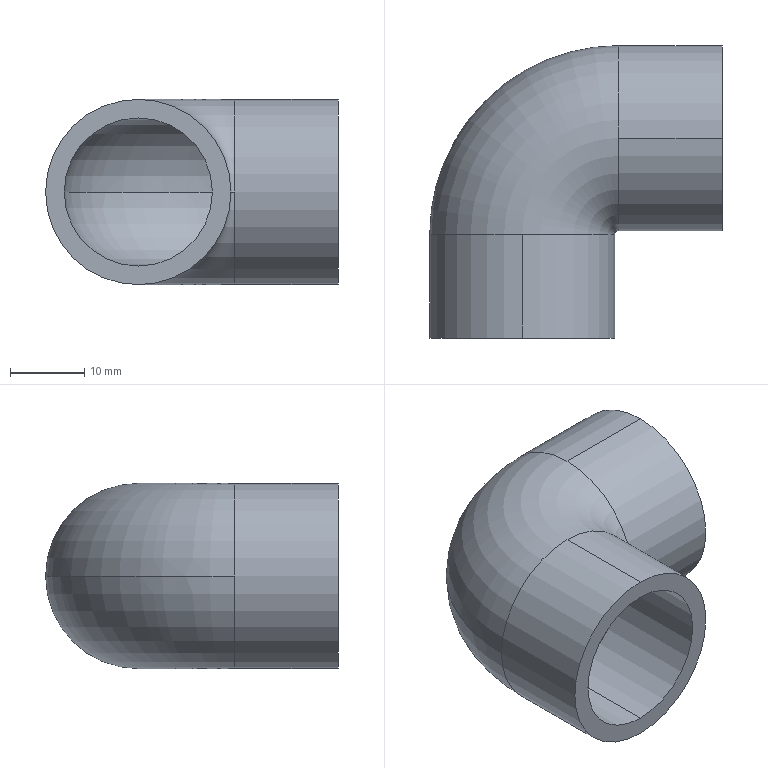Part | SolidWorks | features Sweep 1 | 1 solid | 14 faces | box 39.5 x 39.5 x 25 mm | volume 8557 mm3 | cylinder 8 | torus 4 | plane 2 | commonest cylinder face diameters 20 x4 25 x4
STEP:
#1=CARTESIAN_POINT('',(-10.,14.,0.));
#2=VERTEX_POINT('',#1);
#3=CARTESIAN_POINT('',(0.,14.,10.));
#4=VERTEX_POINT('',#3);
#5=CARTESIAN_POINT('',(0.,14.,0.));
#6=DIRECTION('',(0.,1.,0.));
#7=DIRECTION('',(0.,0.,1.));
#8=AXIS2_PLACEMENT_3D('',#5,#6,#7);
#9=CIRCLE('',#8,10.);
#10=EDGE_CURVE('',#2,#4,#9,.T.);
#11=ORIENTED_EDGE('',*,*,#10,.F.);
#12=CARTESIAN_POINT('',(13.,37.,0.));
#13=VERTEX_POINT('',#12);
#14=CARTESIAN_POINT('',(13.,14.,0.));
#15=DIRECTION('',(0.,0.,-1.));
#16=DIRECTION('',(-1.,0.,0.));
#17=AXIS2_PLACEMENT_3D('',#14,#15,#16);
#18=CIRCLE('',#17,23.);
#19=EDGE_CURVE('',#2,#13,#18,.T.);
#20=ORIENTED_EDGE('',*,*,#19,.T.);
#21=CARTESIAN_POINT('',(13.,27.,10.));
#22=VERTEX_POINT('',#21);
#23=CARTESIAN_POINT('',(13.,27.,0.));
#24=DIRECTION('',(1.,0.,0.));
#25=DIRECTION('',(0.,0.,1.));
#26=AXIS2_PLACEMENT_3D('',#23,#24,#25);
#27=CIRCLE('',#26,10.);
#28=EDGE_CURVE('',#13,#22,#27,.T.);
#29=ORIENTED_EDGE('',*,*,#28,.T.);
#30=CARTESIAN_POINT('',(13.,17.,0.));
#31=VERTEX_POINT('',#30);
#32=CARTESIAN_POINT('',(13.,27.,0.));
#33=DIRECTION('',(1.,0.,0.));
#34=DIRECTION('',(0.,0.,1.));
#35=AXIS2_PLACEMENT_3D('',#32,#33,#34);
#36=CIRCLE('',#35,10.);
#37=EDGE_CURVE('',#22,#31,#36,.T.);
#38=ORIENTED_EDGE('',*,*,#37,.T.);
#39=CARTESIAN_POINT('',(10.,14.,0.));
#40=VERTEX_POINT('',#39);
#41=CARTESIAN_POINT('',(13.,14.,0.));
#42=DIRECTION('',(0.,0.,-1.));
#43=DIRECTION('',(-1.,0.,0.));
#44=AXIS2_PLACEMENT_3D('',#41,#42,#43);
#45=CIRCLE('',#44,3.);
#46=EDGE_CURVE('',#40,#31,#45,.T.);
#47=ORIENTED_EDGE('',*,*,#46,.F.);
#48=CARTESIAN_POINT('',(0.,14.,0.));
#49=DIRECTION('',(0.,1.,0.));
#50=DIRECTION('',(0.,0.,1.));
#51=AXIS2_PLACEMENT_3D('',#48,#49,#50);
#52=CIRCLE('',#51,10.);
#53=EDGE_CURVE('',#4,#40,#52,.T.);
#54=ORIENTED_EDGE('',*,*,#53,.F.);
#55=EDGE_LOOP('',(#11,#20,#29,#38,#47,#54));
#56=FACE_OUTER_BOUND('',#55,.T.);
#57=CARTESIAN_POINT('',(13.,14.,0.));
#58=DIRECTION('',(0.,0.,-1.));
#59=DIRECTION('',(-1.,0.,0.));
#60=AXIS2_PLACEMENT_3D('',#57,#58,#59);
#61=TOROIDAL_SURFACE('',#60,13.,10.);
#62=ADVANCED_FACE('',(#56),#61,.F.);
#63=CARTESIAN_POINT('',(0.,14.,-12.5));
#64=VERTEX_POINT('',#63);
#65=CARTESIAN_POINT('',(-12.5,14.,0.));
#66=VERTEX_POINT('',#65);
#67=CARTESIAN_POINT('',(0.,14.,0.));
#68=DIRECTION('',(0.,1.,0.));
#69=DIRECTION('',(0.,0.,1.));
#70=AXIS2_PLACEMENT_3D('',#67,#68,#69);
#71=CIRCLE('',#70,12.5);
#72=EDGE_CURVE('',#64,#66,#71,.T.);
#73=ORIENTED_EDGE('',*,*,#72,.T.);
#74=CARTESIAN_POINT('',(13.,39.5,0.));
#75=VERTEX_POINT('',#74);
#76=CARTESIAN_POINT('',(13.,14.,0.));
#77=DIRECTION('',(0.,0.,-1.));
#78=DIRECTION('',(-1.,0.,0.));
#79=AXIS2_PLACEMENT_3D('',#76,#77,#78);
#80=CIRCLE('',#79,25.5);
#81=EDGE_CURVE('',#66,#75,#80,.T.);
#82=ORIENTED_EDGE('',*,*,#81,.T.);
#83=CARTESIAN_POINT('',(13.,27.,-12.5));
#84=VERTEX_POINT('',#83);
#85=CARTESIAN_POINT('',(13.,27.,0.));
#86=DIRECTION('',(1.,0.,0.));
#87=DIRECTION('',(0.,0.,1.));
#88=AXIS2_PLACEMENT_3D('',#85,#86,#87);
#89=CIRCLE('',#88,12.5);
#90=EDGE_CURVE('',#84,#75,#89,.T.);
#91=ORIENTED_EDGE('',*,*,#90,.F.);
#92=CARTESIAN_POINT('',(13.,14.5,0.));
#93=VERTEX_POINT('',#92);
#94=CARTESIAN_POINT('',(13.,27.,0.));
#95=DIRECTION('',(1.,0.,0.));
#96=DIRECTION('',(0.,0.,1.));
#97=AXIS2_PLACEMENT_3D('',#94,#95,#96);
#98=CIRCLE('',#97,12.5);
#99=EDGE_CURVE('',#93,#84,#98,.T.);
#100=ORIENTED_EDGE('',*,*,#99,.F.);
#101=CARTESIAN_POINT('',(12.5,14.,0.));
#102=VERTEX_POINT('',#101);
#103=CARTESIAN_POINT('',(13.,14.,0.));
#104=DIRECTION('',(0.,0.,-1.));
#105=DIRECTION('',(-1.,0.,0.));
#106=AXIS2_PLACEMENT_3D('',#103,#104,#105);
#107=CIRCLE('',#106,0.5);
#108=EDGE_CURVE('',#102,#93,#107,.T.);
#109=ORIENTED_EDGE('',*,*,#108,.F.);
#110=CARTESIAN_POINT('',(0.,14.,0.));
#111=DIRECTION('',(0.,1.,0.));
#112=DIRECTION('',(0.,0.,1.));
#113=AXIS2_PLACEMENT_3D('',#110,#111,#112);
#114=CIRCLE('',#113,12.5);
#115=EDGE_CURVE('',#102,#64,#114,.T.);
#116=ORIENTED_EDGE('',*,*,#115,.T.);
#117=EDGE_LOOP('',(#73,#82,#91,#100,#109,#116));
#118=FACE_OUTER_BOUND('',#117,.T.);
#119=CARTESIAN_POINT('',(13.,14.,0.));
#120=DIRECTION('',(0.,0.,-1.));
#121=DIRECTION('',(-1.,0.,0.));
#122=AXIS2_PLACEMENT_3D('',#119,#120,#121);
#123=TOROIDAL_SURFACE('',#122,13.,12.5);
#124=ADVANCED_FACE('',(#118),#123,.T.);
#125=CARTESIAN_POINT('',(0.,14.,12.5));
#126=VERTEX_POINT('',#125);
#127=CARTESIAN_POINT('',(0.,14.,0.));
#128=DIRECTION('',(0.,1.,0.));
#129=DIRECTION('',(0.,0.,1.));
#130=AXIS2_PLACEMENT_3D('',#127,#128,#129);
#131=CIRCLE('',#130,12.5);
#132=EDGE_CURVE('',#126,#102,#131,.T.);
#133=ORIENTED_EDGE('',*,*,#132,.F.);
#134=CARTESIAN_POINT('',(0.,0.,12.5));
#135=VERTEX_POINT('',#134);
#136=CARTESIAN_POINT('',(0.,14.,12.5));
#137=DIRECTION('',(0.,-1.,0.));
#138=VECTOR('',#137,1000.);
#139=LINE('',#136,#138);
#140=EDGE_CURVE('',#126,#135,#139,.T.);
#141=ORIENTED_EDGE('',*,*,#140,.T.);
#142=CARTESIAN_POINT('',(0.,0.,-12.5));
#143=VERTEX_POINT('',#142);
#144=CARTESIAN_POINT('',(0.,0.,0.));
#145=DIRECTION('',(0.,1.,0.));
#146=DIRECTION('',(0.,0.,1.));
#147=AXIS2_PLACEMENT_3D('',#144,#145,#146);
#148=CIRCLE('',#147,12.5);
#149=EDGE_CURVE('',#135,#143,#148,.T.);
#150=ORIENTED_EDGE('',*,*,#149,.T.);
#151=CARTESIAN_POINT('',(0.,14.,-12.5));
#152=DIRECTION('',(0.,-1.,0.));
#153=VECTOR('',#152,1000.);
#154=LINE('',#151,#153);
#155=EDGE_CURVE('',#64,#143,#154,.T.);
#156=ORIENTED_EDGE('',*,*,#155,.F.);
#157=ORIENTED_EDGE('',*,*,#115,.F.);
#158=EDGE_LOOP('',(#133,#141,#150,#156,#157));
#159=FACE_OUTER_BOUND('',#158,.T.);
#160=CARTESIAN_POINT('',(0.,14.,0.));
#161=DIRECTION('',(0.,-1.,0.));
#162=DIRECTION('',(0.,0.,-1.));
#163=AXIS2_PLACEMENT_3D('',#160,#161,#162);
#164=CYLINDRICAL_SURFACE('',#163,12.5);
#165=ADVANCED_FACE('',(#159),#164,.T.);
#166=CARTESIAN_POINT('',(0.,14.,-10.));
#167=VERTEX_POINT('',#166);
#168=CARTESIAN_POINT('',(0.,14.,0.));
#169=DIRECTION('',(0.,1.,0.));
#170=DIRECTION('',(0.,0.,1.));
#171=AXIS2_PLACEMENT_3D('',#168,#169,#170);
#172=CIRCLE('',#171,10.);
#173=EDGE_CURVE('',#167,#2,#172,.T.);
#174=ORIENTED_EDGE('',*,*,#173,.T.);
#175=ORIENTED_EDGE('',*,*,#10,.T.);
#176=CARTESIAN_POINT('',(0.,0.,10.));
#177=VERTEX_POINT('',#176);
#178=CARTESIAN_POINT('',(0.,14.,10.));
#179=DIRECTION('',(0.,-1.,0.));
#180=VECTOR('',#179,1000.);
#181=LINE('',#178,#180);
#182=EDGE_CURVE('',#4,#177,#181,.T.);
#183=ORIENTED_EDGE('',*,*,#182,.T.);
#184=CARTESIAN_POINT('',(0.,0.,-10.));
#185=VERTEX_POINT('',#184);
#186=CARTESIAN_POINT('',(0.,0.,0.));
#187=DIRECTION('',(0.,1.,0.));
#188=DIRECTION('',(0.,0.,1.));
#189=AXIS2_PLACEMENT_3D('',#186,#187,#188);
#190=CIRCLE('',#189,10.);
#191=EDGE_CURVE('',#185,#177,#190,.T.);
#192=ORIENTED_EDGE('',*,*,#191,.F.);
#193=CARTESIAN_POINT('',(0.,14.,-10.));
#194=DIRECTION('',(0.,-1.,0.));
#195=VECTOR('',#194,1000.);
#196=LINE('',#193,#195);
#197=EDGE_CURVE('',#167,#185,#196,.T.);
#198=ORIENTED_EDGE('',*,*,#197,.F.);
#199=EDGE_LOOP('',(#174,#175,#183,#192,#198));
#200=FACE_OUTER_BOUND('',#199,.T.);
#201=CARTESIAN_POINT('',(0.,14.,0.));
#202=DIRECTION('',(0.,-1.,0.));
#203=DIRECTION('',(0.,0.,-1.));
#204=AXIS2_PLACEMENT_3D('',#201,#202,#203);
#205=CYLINDRICAL_SURFACE('',#204,10.);
#206=ADVANCED_FACE('',(#200),#205,.F.);
#207=ORIENTED_EDGE('',*,*,#37,.F.);
#208=CARTESIAN_POINT('',(27.,27.,10.));
#209=VERTEX_POINT('',#208);
#210=CARTESIAN_POINT('',(13.,27.,10.));
#211=DIRECTION('',(1.,0.,0.));
#212=VECTOR('',#211,1000.);
#213=LINE('',#210,#212);
#214=EDGE_CURVE('',#22,#209,#213,.T.);
#215=ORIENTED_EDGE('',*,*,#214,.T.);
#216=CARTESIAN_POINT('',(27.,27.,-10.));
#217=VERTEX_POINT('',#216);
#218=CARTESIAN_POINT('',(27.,27.,0.));
#219=DIRECTION('',(1.,0.,0.));
#220=DIRECTION('',(0.,0.,1.));
#221=AXIS2_PLACEMENT_3D('',#218,#219,#220);
#222=CIRCLE('',#221,10.);
#223=EDGE_CURVE('',#209,#217,#222,.T.);
#224=ORIENTED_EDGE('',*,*,#223,.T.);
#225=CARTESIAN_POINT('',(13.,27.,-10.));
#226=VERTEX_POINT('',#225);
#227=CARTESIAN_POINT('',(13.,27.,-10.));
#228=DIRECTION('',(1.,0.,0.));
#229=VECTOR('',#228,1000.);
#230=LINE('',#227,#229);
#231=EDGE_CURVE('',#226,#217,#230,.T.);
#232=ORIENTED_EDGE('',*,*,#231,.F.);
#233=CARTESIAN_POINT('',(13.,27.,0.));
#234=DIRECTION('',(1.,0.,0.));
#235=DIRECTION('',(0.,0.,1.));
#236=AXIS2_PLACEMENT_3D('',#233,#234,#235);
#237=CIRCLE('',#236,10.);
#238=EDGE_CURVE('',#31,#226,#237,.T.);
#239=ORIENTED_EDGE('',*,*,#238,.F.);
#240=EDGE_LOOP('',(#207,#215,#224,#232,#239));
#241=FACE_OUTER_BOUND('',#240,.T.);
#242=CARTESIAN_POINT('',(13.,27.,0.));
#243=DIRECTION('',(1.,0.,0.));
#244=DIRECTION('',(0.,0.,-1.));
#245=AXIS2_PLACEMENT_3D('',#242,#243,#244);
#246=CYLINDRICAL_SURFACE('',#245,10.);
#247=ADVANCED_FACE('',(#241),#246,.F.);
#248=ORIENTED_EDGE('',*,*,#90,.T.);
#249=CARTESIAN_POINT('',(13.,27.,12.5));
#250=VERTEX_POINT('',#249);
#251=CARTESIAN_POINT('',(13.,27.,0.));
#252=DIRECTION('',(1.,0.,0.));
#253=DIRECTION('',(0.,0.,1.));
#254=AXIS2_PLACEMENT_3D('',#251,#252,#253);
#255=CIRCLE('',#254,12.5);
#256=EDGE_CURVE('',#75,#250,#255,.T.);
#257=ORIENTED_EDGE('',*,*,#256,.T.);
#258=CARTESIAN_POINT('',(27.,27.,12.5));
#259=VERTEX_POINT('',#258);
#260=CARTESIAN_POINT('',(13.,27.,12.5));
#261=DIRECTION('',(1.,0.,0.));
#262=VECTOR('',#261,1000.);
#263=LINE('',#260,#262);
#264=EDGE_CURVE('',#250,#259,#263,.T.);
#265=ORIENTED_EDGE('',*,*,#264,.T.);
#266=CARTESIAN_POINT('',(27.,27.,-12.5));
#267=VERTEX_POINT('',#266);
#268=CARTESIAN_POINT('',(27.,27.,0.));
#269=DIRECTION('',(1.,0.,0.));
#270=DIRECTION('',(0.,0.,1.));
#271=AXIS2_PLACEMENT_3D('',#268,#269,#270);
#272=CIRCLE('',#271,12.5);
#273=EDGE_CURVE('',#267,#259,#272,.T.);
#274=ORIENTED_EDGE('',*,*,#273,.F.);
#275=CARTESIAN_POINT('',(13.,27.,-12.5));
#276=DIRECTION('',(1.,0.,0.));
#277=VECTOR('',#276,1000.);
#278=LINE('',#275,#277);
#279=EDGE_CURVE('',#84,#267,#278,.T.);
#280=ORIENTED_EDGE('',*,*,#279,.F.);
#281=EDGE_LOOP('',(#248,#257,#265,#274,#280));
#282=FACE_OUTER_BOUND('',#281,.T.);
#283=CARTESIAN_POINT('',(13.,27.,0.));
#284=DIRECTION('',(1.,0.,0.));
#285=DIRECTION('',(0.,0.,-1.));
#286=AXIS2_PLACEMENT_3D('',#283,#284,#285);
#287=CYLINDRICAL_SURFACE('',#286,12.5);
#288=ADVANCED_FACE('',(#282),#287,.T.);
#289=ORIENTED_EDGE('',*,*,#264,.F.);
#290=CARTESIAN_POINT('',(13.,27.,0.));
#291=DIRECTION('',(1.,0.,0.));
#292=DIRECTION('',(0.,0.,1.));
#293=AXIS2_PLACEMENT_3D('',#290,#291,#292);
#294=CIRCLE('',#293,12.5);
#295=EDGE_CURVE('',#250,#93,#294,.T.);
#296=ORIENTED_EDGE('',*,*,#295,.T.);
#297=ORIENTED_EDGE('',*,*,#99,.T.);
#298=ORIENTED_EDGE('',*,*,#279,.T.);
#299=CARTESIAN_POINT('',(27.,27.,0.));
#300=DIRECTION('',(1.,0.,0.));
#301=DIRECTION('',(0.,0.,1.));
#302=AXIS2_PLACEMENT_3D('',#299,#300,#301);
#303=CIRCLE('',#302,12.5);
#304=EDGE_CURVE('',#259,#267,#303,.T.);
#305=ORIENTED_EDGE('',*,*,#304,.F.);
#306=EDGE_LOOP('',(#289,#296,#297,#298,#305));
#307=FACE_OUTER_BOUND('',#306,.T.);
#308=CARTESIAN_POINT('',(13.,27.,0.));
#309=DIRECTION('',(1.,0.,0.));
#310=DIRECTION('',(0.,0.,-1.));
#311=AXIS2_PLACEMENT_3D('',#308,#309,#310);
#312=CYLINDRICAL_SURFACE('',#311,12.5);
#313=ADVANCED_FACE('',(#307),#312,.T.);
#314=ORIENTED_EDGE('',*,*,#214,.F.);
#315=ORIENTED_EDGE('',*,*,#28,.F.);
#316=CARTESIAN_POINT('',(13.,27.,0.));
#317=DIRECTION('',(1.,0.,0.));
#318=DIRECTION('',(0.,0.,1.));
#319=AXIS2_PLACEMENT_3D('',#316,#317,#318);
#320=CIRCLE('',#319,10.);
#321=EDGE_CURVE('',#226,#13,#320,.T.);
#322=ORIENTED_EDGE('',*,*,#321,.F.);
#323=ORIENTED_EDGE('',*,*,#231,.T.);
#324=CARTESIAN_POINT('',(27.,27.,0.));
#325=DIRECTION('',(1.,0.,0.));
#326=DIRECTION('',(0.,0.,1.));
#327=AXIS2_PLACEMENT_3D('',#324,#325,#326);
#328=CIRCLE('',#327,10.);
#329=EDGE_CURVE('',#217,#209,#328,.T.);
#330=ORIENTED_EDGE('',*,*,#329,.T.);
#331=EDGE_LOOP('',(#314,#315,#322,#323,#330));
#332=FACE_OUTER_BOUND('',#331,.T.);
#333=CARTESIAN_POINT('',(13.,27.,0.));
#334=DIRECTION('',(1.,0.,0.));
#335=DIRECTION('',(0.,0.,-1.));
#336=AXIS2_PLACEMENT_3D('',#333,#334,#335);
#337=CYLINDRICAL_SURFACE('',#336,10.);
#338=ADVANCED_FACE('',(#332),#337,.F.);
#339=ORIENTED_EDGE('',*,*,#81,.F.);
#340=CARTESIAN_POINT('',(0.,14.,0.));
#341=DIRECTION('',(0.,1.,0.));
#342=DIRECTION('',(0.,0.,1.));
#343=AXIS2_PLACEMENT_3D('',#340,#341,#342);
#344=CIRCLE('',#343,12.5);
#345=EDGE_CURVE('',#66,#126,#344,.T.);
#346=ORIENTED_EDGE('',*,*,#345,.T.);
#347=ORIENTED_EDGE('',*,*,#132,.T.);
#348=ORIENTED_EDGE('',*,*,#108,.T.);
#349=ORIENTED_EDGE('',*,*,#295,.F.);
#350=ORIENTED_EDGE('',*,*,#256,.F.);
#351=EDGE_LOOP('',(#339,#346,#347,#348,#349,#350));
#352=FACE_OUTER_BOUND('',#351,.T.);
#353=CARTESIAN_POINT('',(13.,14.,0.));
#354=DIRECTION('',(0.,0.,-1.));
#355=DIRECTION('',(-1.,0.,0.));
#356=AXIS2_PLACEMENT_3D('',#353,#354,#355);
#357=TOROIDAL_SURFACE('',#356,13.,12.5);
#358=ADVANCED_FACE('',(#352),#357,.T.);
#359=ORIENTED_EDGE('',*,*,#19,.F.);
#360=ORIENTED_EDGE('',*,*,#173,.F.);
#361=CARTESIAN_POINT('',(0.,14.,0.));
#362=DIRECTION('',(0.,1.,0.));
#363=DIRECTION('',(0.,0.,1.));
#364=AXIS2_PLACEMENT_3D('',#361,#362,#363);
#365=CIRCLE('',#364,10.);
#366=EDGE_CURVE('',#40,#167,#365,.T.);
#367=ORIENTED_EDGE('',*,*,#366,.F.);
#368=ORIENTED_EDGE('',*,*,#46,.T.);
#369=ORIENTED_EDGE('',*,*,#238,.T.);
#370=ORIENTED_EDGE('',*,*,#321,.T.);
#371=EDGE_LOOP('',(#359,#360,#367,#368,#369,#370));
#372=FACE_OUTER_BOUND('',#371,.T.);
#373=CARTESIAN_POINT('',(13.,14.,0.));
#374=DIRECTION('',(0.,0.,-1.));
#375=DIRECTION('',(-1.,0.,0.));
#376=AXIS2_PLACEMENT_3D('',#373,#374,#375);
#377=TOROIDAL_SURFACE('',#376,13.,10.);
#378=ADVANCED_FACE('',(#372),#377,.F.);
#379=ORIENTED_EDGE('',*,*,#182,.F.);
#380=ORIENTED_EDGE('',*,*,#53,.T.);
#381=ORIENTED_EDGE('',*,*,#366,.T.);
#382=ORIENTED_EDGE('',*,*,#197,.T.);
#383=CARTESIAN_POINT('',(0.,0.,0.));
#384=DIRECTION('',(0.,1.,0.));
#385=DIRECTION('',(0.,0.,1.));
#386=AXIS2_PLACEMENT_3D('',#383,#384,#385);
#387=CIRCLE('',#386,10.);
#388=EDGE_CURVE('',#177,#185,#387,.T.);
#389=ORIENTED_EDGE('',*,*,#388,.F.);
#390=EDGE_LOOP('',(#379,#380,#381,#382,#389));
#391=FACE_OUTER_BOUND('',#390,.T.);
#392=CARTESIAN_POINT('',(0.,14.,0.));
#393=DIRECTION('',(0.,-1.,0.));
#394=DIRECTION('',(0.,0.,-1.));
#395=AXIS2_PLACEMENT_3D('',#392,#393,#394);
#396=CYLINDRICAL_SURFACE('',#395,10.);
#397=ADVANCED_FACE('',(#391),#396,.F.);
#398=ORIENTED_EDGE('',*,*,#140,.F.);
#399=ORIENTED_EDGE('',*,*,#345,.F.);
#400=ORIENTED_EDGE('',*,*,#72,.F.);
#401=ORIENTED_EDGE('',*,*,#155,.T.);
#402=CARTESIAN_POINT('',(0.,0.,0.));
#403=DIRECTION('',(0.,1.,0.));
#404=DIRECTION('',(0.,0.,1.));
#405=AXIS2_PLACEMENT_3D('',#402,#403,#404);
#406=CIRCLE('',#405,12.5);
#407=EDGE_CURVE('',#143,#135,#406,.T.);
#408=ORIENTED_EDGE('',*,*,#407,.T.);
#409=EDGE_LOOP('',(#398,#399,#400,#401,#408));
#410=FACE_OUTER_BOUND('',#409,.T.);
#411=CARTESIAN_POINT('',(0.,14.,0.));
#412=DIRECTION('',(0.,-1.,0.));
#413=DIRECTION('',(0.,0.,-1.));
#414=AXIS2_PLACEMENT_3D('',#411,#412,#413);
#415=CYLINDRICAL_SURFACE('',#414,12.5);
#416=ADVANCED_FACE('',(#410),#415,.T.);
#417=ORIENTED_EDGE('',*,*,#329,.F.);
#418=ORIENTED_EDGE('',*,*,#223,.F.);
#419=EDGE_LOOP('',(#417,#418));
#420=FACE_BOUND('',#419,.T.);
#421=ORIENTED_EDGE('',*,*,#273,.T.);
#422=ORIENTED_EDGE('',*,*,#304,.T.);
#423=EDGE_LOOP('',(#421,#422));
#424=FACE_OUTER_BOUND('',#423,.T.);
#425=CARTESIAN_POINT('',(27.,27.,0.));
#426=DIRECTION('',(1.,0.,0.));
#427=DIRECTION('',(0.,0.,1.));
#428=AXIS2_PLACEMENT_3D('',#425,#426,#427);
#429=PLANE('',#428);
#430=ADVANCED_FACE('',(#420,#424),#429,.T.);
#431=ORIENTED_EDGE('',*,*,#191,.T.);
#432=ORIENTED_EDGE('',*,*,#388,.T.);
#433=EDGE_LOOP('',(#431,#432));
#434=FACE_BOUND('',#433,.T.);
#435=ORIENTED_EDGE('',*,*,#407,.F.);
#436=ORIENTED_EDGE('',*,*,#149,.F.);
#437=EDGE_LOOP('',(#435,#436));
#438=FACE_OUTER_BOUND('',#437,.T.);
#439=CARTESIAN_POINT('',(0.,0.,0.));
#440=DIRECTION('',(0.,1.,0.));
#441=DIRECTION('',(0.,0.,1.));
#442=AXIS2_PLACEMENT_3D('',#439,#440,#441);
#443=PLANE('',#442);
#444=ADVANCED_FACE('',(#434,#438),#443,.F.);
#445=CLOSED_SHELL('',(#62,#124,#165,#206,#247,#288,#313,#338,#358,#378,#397,#416,#430,#444));
#446=MANIFOLD_SOLID_BREP('',#445);
#447=CARTESIAN_POINT('',(0.,0.,0.));
#448=DIRECTION('',(0.,0.,1.));
#449=DIRECTION('',(1.,0.,0.));
#450=AXIS2_PLACEMENT_3D('',#447,#448,#449);
#451=(LENGTH_UNIT()NAMED_UNIT(*)SI_UNIT(.MILLI.,.METRE.));
#452=UNCERTAINTY_MEASURE_WITH_UNIT(LENGTH_MEASURE(0.00001),#451,'','');
#453=(NAMED_UNIT(*)PLANE_ANGLE_UNIT()SI_UNIT($,.RADIAN.));
#454=(NAMED_UNIT(*)SI_UNIT($,.STERADIAN.)SOLID_ANGLE_UNIT());
#455=(GEOMETRIC_REPRESENTATION_CONTEXT(3)GLOBAL_UNCERTAINTY_ASSIGNED_CONTEXT((#452))GLOBAL_UNIT_ASSIGNED_CONTEXT((#451,#453,#454))REPRESENTATION_CONTEXT('',''));
#456=ADVANCED_BREP_SHAPE_REPRESENTATION('',(#446,#450),#455);